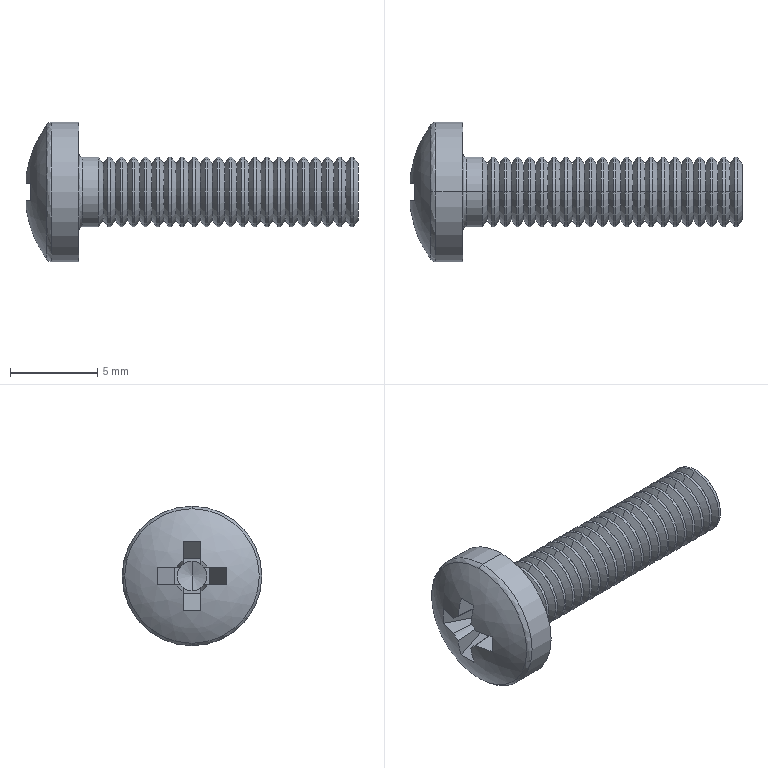Part | SolidWorks | features BaseBody 1 | 1 solid | 161 faces | box 19.021 x 8 x 8 mm | volume 284.545 mm3 | cone 92 | cylinder 46 | plane 18 | spline 5 | commonest cylinder face diameters 4 x44 8 x2